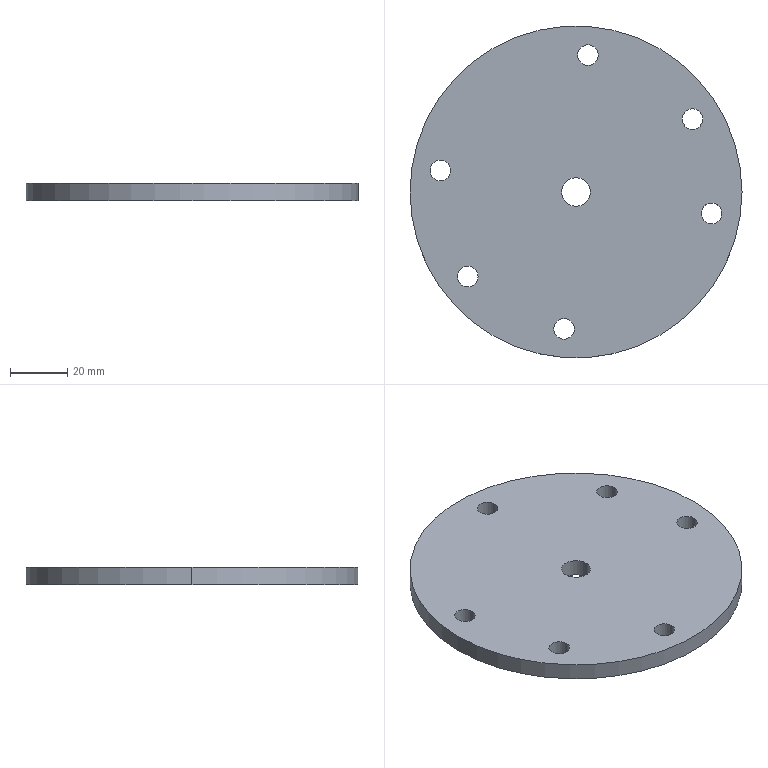Part | SolidWorks | features FlatPattern 1, SMBaseFlange 1, SheetMetal 1 | 1 solid | 18 faces | box 116 x 116 x 6 mm | volume 61473 mm3 | cylinder 16 | plane 2 | commonest cylinder face diameters 7.2 x12 10 x2 116 x2
STEP:
#1=CARTESIAN_POINT('',(-5.,0.,6.));
#2=VERTEX_POINT('',#1);
#3=CARTESIAN_POINT('',(5.,0.,6.));
#4=VERTEX_POINT('',#3);
#5=CARTESIAN_POINT('',(0.,0.,6.));
#6=DIRECTION('',(0.,0.,1.));
#7=DIRECTION('',(1.,0.,0.));
#8=AXIS2_PLACEMENT_3D('',#5,#6,#7);
#9=CIRCLE('',#8,5.);
#10=EDGE_CURVE('',#2,#4,#9,.T.);
#11=ORIENTED_EDGE('',*,*,#10,.T.);
#12=CARTESIAN_POINT('',(5.,0.,0.));
#13=VERTEX_POINT('',#12);
#14=CARTESIAN_POINT('',(5.,0.,6.));
#15=DIRECTION('',(0.,0.,-1.));
#16=VECTOR('',#15,1000.);
#17=LINE('',#14,#16);
#18=EDGE_CURVE('',#4,#13,#17,.T.);
#19=ORIENTED_EDGE('',*,*,#18,.T.);
#20=CARTESIAN_POINT('',(-5.,0.,0.));
#21=VERTEX_POINT('',#20);
#22=CARTESIAN_POINT('',(0.,0.,0.));
#23=DIRECTION('',(0.,0.,1.));
#24=DIRECTION('',(1.,0.,0.));
#25=AXIS2_PLACEMENT_3D('',#22,#23,#24);
#26=CIRCLE('',#25,5.);
#27=EDGE_CURVE('',#21,#13,#26,.T.);
#28=ORIENTED_EDGE('',*,*,#27,.F.);
#29=CARTESIAN_POINT('',(-5.,0.,6.));
#30=DIRECTION('',(0.,0.,-1.));
#31=VECTOR('',#30,1000.);
#32=LINE('',#29,#31);
#33=EDGE_CURVE('',#2,#21,#32,.T.);
#34=ORIENTED_EDGE('',*,*,#33,.F.);
#35=EDGE_LOOP('',(#11,#19,#28,#34));
#36=FACE_OUTER_BOUND('',#35,.T.);
#37=CARTESIAN_POINT('',(0.,0.,6.));
#38=DIRECTION('',(0.,0.,-1.));
#39=DIRECTION('',(-1.,0.,0.));
#40=AXIS2_PLACEMENT_3D('',#37,#38,#39);
#41=CYLINDRICAL_SURFACE('',#40,5.);
#42=ADVANCED_FACE('',(#36),#41,.F.);
#43=CARTESIAN_POINT('',(-7.783,-47.817,6.));
#44=VERTEX_POINT('',#43);
#45=CARTESIAN_POINT('',(-0.5835,-47.817,6.));
#46=VERTEX_POINT('',#45);
#47=CARTESIAN_POINT('',(-4.183,-47.817,6.));
#48=DIRECTION('',(0.,0.,1.));
#49=DIRECTION('',(1.,0.,0.));
#50=AXIS2_PLACEMENT_3D('',#47,#48,#49);
#51=CIRCLE('',#50,3.6);
#52=EDGE_CURVE('',#44,#46,#51,.T.);
#53=ORIENTED_EDGE('',*,*,#52,.T.);
#54=CARTESIAN_POINT('',(-0.5835,-47.817,0.));
#55=VERTEX_POINT('',#54);
#56=CARTESIAN_POINT('',(-0.5835,-47.817,6.));
#57=DIRECTION('',(0.,0.,-1.));
#58=VECTOR('',#57,1000.);
#59=LINE('',#56,#58);
#60=EDGE_CURVE('',#46,#55,#59,.T.);
#61=ORIENTED_EDGE('',*,*,#60,.T.);
#62=CARTESIAN_POINT('',(-7.783,-47.817,0.));
#63=VERTEX_POINT('',#62);
#64=CARTESIAN_POINT('',(-4.183,-47.817,0.));
#65=DIRECTION('',(0.,0.,1.));
#66=DIRECTION('',(1.,0.,0.));
#67=AXIS2_PLACEMENT_3D('',#64,#65,#66);
#68=CIRCLE('',#67,3.6);
#69=EDGE_CURVE('',#63,#55,#68,.T.);
#70=ORIENTED_EDGE('',*,*,#69,.F.);
#71=CARTESIAN_POINT('',(-7.783,-47.817,6.));
#72=DIRECTION('',(0.,0.,-1.));
#73=VECTOR('',#72,1000.);
#74=LINE('',#71,#73);
#75=EDGE_CURVE('',#44,#63,#74,.T.);
#76=ORIENTED_EDGE('',*,*,#75,.F.);
#77=EDGE_LOOP('',(#53,#61,#70,#76));
#78=FACE_OUTER_BOUND('',#77,.T.);
#79=CARTESIAN_POINT('',(-4.183,-47.817,6.));
#80=DIRECTION('',(0.,0.,-1.));
#81=DIRECTION('',(-1.,0.,0.));
#82=AXIS2_PLACEMENT_3D('',#79,#80,#81);
#83=CYLINDRICAL_SURFACE('',#82,3.6);
#84=ADVANCED_FACE('',(#78),#83,.F.);
#85=CARTESIAN_POINT('',(43.809,-7.509,6.));
#86=VERTEX_POINT('',#85);
#87=CARTESIAN_POINT('',(51.009,-7.509,6.));
#88=VERTEX_POINT('',#87);
#89=CARTESIAN_POINT('',(47.409,-7.509,6.));
#90=DIRECTION('',(0.,0.,1.));
#91=DIRECTION('',(1.,0.,0.));
#92=AXIS2_PLACEMENT_3D('',#89,#90,#91);
#93=CIRCLE('',#92,3.6);
#94=EDGE_CURVE('',#86,#88,#93,.T.);
#95=ORIENTED_EDGE('',*,*,#94,.T.);
#96=CARTESIAN_POINT('',(51.009,-7.509,0.));
#97=VERTEX_POINT('',#96);
#98=CARTESIAN_POINT('',(51.009,-7.509,6.));
#99=DIRECTION('',(0.,0.,-1.));
#100=VECTOR('',#99,1000.);
#101=LINE('',#98,#100);
#102=EDGE_CURVE('',#88,#97,#101,.T.);
#103=ORIENTED_EDGE('',*,*,#102,.T.);
#104=CARTESIAN_POINT('',(43.809,-7.509,0.));
#105=VERTEX_POINT('',#104);
#106=CARTESIAN_POINT('',(47.409,-7.509,0.));
#107=DIRECTION('',(0.,0.,1.));
#108=DIRECTION('',(1.,0.,0.));
#109=AXIS2_PLACEMENT_3D('',#106,#107,#108);
#110=CIRCLE('',#109,3.6);
#111=EDGE_CURVE('',#105,#97,#110,.T.);
#112=ORIENTED_EDGE('',*,*,#111,.F.);
#113=CARTESIAN_POINT('',(43.809,-7.509,6.));
#114=DIRECTION('',(0.,0.,-1.));
#115=VECTOR('',#114,1000.);
#116=LINE('',#113,#115);
#117=EDGE_CURVE('',#86,#105,#116,.T.);
#118=ORIENTED_EDGE('',*,*,#117,.F.);
#119=EDGE_LOOP('',(#95,#103,#112,#118));
#120=FACE_OUTER_BOUND('',#119,.T.);
#121=CARTESIAN_POINT('',(47.409,-7.509,6.));
#122=DIRECTION('',(0.,0.,-1.));
#123=DIRECTION('',(-1.,0.,0.));
#124=AXIS2_PLACEMENT_3D('',#121,#122,#123);
#125=CYLINDRICAL_SURFACE('',#124,3.6);
#126=ADVANCED_FACE('',(#120),#125,.F.);
#127=CARTESIAN_POINT('',(37.106,25.436,6.));
#128=VERTEX_POINT('',#127);
#129=CARTESIAN_POINT('',(44.306,25.436,6.));
#130=VERTEX_POINT('',#129);
#131=CARTESIAN_POINT('',(40.706,25.436,6.));
#132=DIRECTION('',(0.,0.,1.));
#133=DIRECTION('',(1.,0.,0.));
#134=AXIS2_PLACEMENT_3D('',#131,#132,#133);
#135=CIRCLE('',#134,3.6);
#136=EDGE_CURVE('',#128,#130,#135,.T.);
#137=ORIENTED_EDGE('',*,*,#136,.T.);
#138=CARTESIAN_POINT('',(44.306,25.436,0.));
#139=VERTEX_POINT('',#138);
#140=CARTESIAN_POINT('',(44.306,25.436,6.));
#141=DIRECTION('',(0.,0.,-1.));
#142=VECTOR('',#141,1000.);
#143=LINE('',#140,#142);
#144=EDGE_CURVE('',#130,#139,#143,.T.);
#145=ORIENTED_EDGE('',*,*,#144,.T.);
#146=CARTESIAN_POINT('',(37.106,25.436,0.));
#147=VERTEX_POINT('',#146);
#148=CARTESIAN_POINT('',(40.706,25.436,0.));
#149=DIRECTION('',(0.,0.,1.));
#150=DIRECTION('',(1.,0.,0.));
#151=AXIS2_PLACEMENT_3D('',#148,#149,#150);
#152=CIRCLE('',#151,3.6);
#153=EDGE_CURVE('',#147,#139,#152,.T.);
#154=ORIENTED_EDGE('',*,*,#153,.F.);
#155=CARTESIAN_POINT('',(37.106,25.436,6.));
#156=DIRECTION('',(0.,0.,-1.));
#157=VECTOR('',#156,1000.);
#158=LINE('',#155,#157);
#159=EDGE_CURVE('',#128,#147,#158,.T.);
#160=ORIENTED_EDGE('',*,*,#159,.F.);
#161=EDGE_LOOP('',(#137,#145,#154,#160));
#162=FACE_OUTER_BOUND('',#161,.T.);
#163=CARTESIAN_POINT('',(40.706,25.436,6.));
#164=DIRECTION('',(0.,0.,-1.));
#165=DIRECTION('',(-1.,0.,0.));
#166=AXIS2_PLACEMENT_3D('',#163,#164,#165);
#167=CYLINDRICAL_SURFACE('',#166,3.6);
#168=ADVANCED_FACE('',(#162),#167,.F.);
#169=CARTESIAN_POINT('',(0.5835,47.817,6.));
#170=VERTEX_POINT('',#169);
#171=CARTESIAN_POINT('',(7.783,47.817,6.));
#172=VERTEX_POINT('',#171);
#173=CARTESIAN_POINT('',(4.183,47.817,6.));
#174=DIRECTION('',(0.,0.,1.));
#175=DIRECTION('',(1.,0.,0.));
#176=AXIS2_PLACEMENT_3D('',#173,#174,#175);
#177=CIRCLE('',#176,3.6);
#178=EDGE_CURVE('',#170,#172,#177,.T.);
#179=ORIENTED_EDGE('',*,*,#178,.T.);
#180=CARTESIAN_POINT('',(7.783,47.817,0.));
#181=VERTEX_POINT('',#180);
#182=CARTESIAN_POINT('',(7.783,47.817,6.));
#183=DIRECTION('',(0.,0.,-1.));
#184=VECTOR('',#183,1000.);
#185=LINE('',#182,#184);
#186=EDGE_CURVE('',#172,#181,#185,.T.);
#187=ORIENTED_EDGE('',*,*,#186,.T.);
#188=CARTESIAN_POINT('',(0.5835,47.817,0.));
#189=VERTEX_POINT('',#188);
#190=CARTESIAN_POINT('',(4.183,47.817,0.));
#191=DIRECTION('',(0.,0.,1.));
#192=DIRECTION('',(1.,0.,0.));
#193=AXIS2_PLACEMENT_3D('',#190,#191,#192);
#194=CIRCLE('',#193,3.6);
#195=EDGE_CURVE('',#189,#181,#194,.T.);
#196=ORIENTED_EDGE('',*,*,#195,.F.);
#197=CARTESIAN_POINT('',(0.5835,47.817,6.));
#198=DIRECTION('',(0.,0.,-1.));
#199=VECTOR('',#198,1000.);
#200=LINE('',#197,#199);
#201=EDGE_CURVE('',#170,#189,#200,.T.);
#202=ORIENTED_EDGE('',*,*,#201,.F.);
#203=EDGE_LOOP('',(#179,#187,#196,#202));
#204=FACE_OUTER_BOUND('',#203,.T.);
#205=CARTESIAN_POINT('',(4.183,47.817,6.));
#206=DIRECTION('',(0.,0.,-1.));
#207=DIRECTION('',(-1.,0.,0.));
#208=AXIS2_PLACEMENT_3D('',#205,#206,#207);
#209=CYLINDRICAL_SURFACE('',#208,3.6);
#210=ADVANCED_FACE('',(#204),#209,.F.);
#211=CARTESIAN_POINT('',(-51.009,7.509,6.));
#212=VERTEX_POINT('',#211);
#213=CARTESIAN_POINT('',(-43.809,7.509,6.));
#214=VERTEX_POINT('',#213);
#215=CARTESIAN_POINT('',(-47.409,7.509,6.));
#216=DIRECTION('',(0.,0.,1.));
#217=DIRECTION('',(1.,0.,0.));
#218=AXIS2_PLACEMENT_3D('',#215,#216,#217);
#219=CIRCLE('',#218,3.6);
#220=EDGE_CURVE('',#212,#214,#219,.T.);
#221=ORIENTED_EDGE('',*,*,#220,.T.);
#222=CARTESIAN_POINT('',(-43.809,7.509,0.));
#223=VERTEX_POINT('',#222);
#224=CARTESIAN_POINT('',(-43.809,7.509,6.));
#225=DIRECTION('',(0.,0.,-1.));
#226=VECTOR('',#225,1000.);
#227=LINE('',#224,#226);
#228=EDGE_CURVE('',#214,#223,#227,.T.);
#229=ORIENTED_EDGE('',*,*,#228,.T.);
#230=CARTESIAN_POINT('',(-51.009,7.509,0.));
#231=VERTEX_POINT('',#230);
#232=CARTESIAN_POINT('',(-47.409,7.509,0.));
#233=DIRECTION('',(0.,0.,1.));
#234=DIRECTION('',(1.,0.,0.));
#235=AXIS2_PLACEMENT_3D('',#232,#233,#234);
#236=CIRCLE('',#235,3.6);
#237=EDGE_CURVE('',#231,#223,#236,.T.);
#238=ORIENTED_EDGE('',*,*,#237,.F.);
#239=CARTESIAN_POINT('',(-51.009,7.509,6.));
#240=DIRECTION('',(0.,0.,-1.));
#241=VECTOR('',#240,1000.);
#242=LINE('',#239,#241);
#243=EDGE_CURVE('',#212,#231,#242,.T.);
#244=ORIENTED_EDGE('',*,*,#243,.F.);
#245=EDGE_LOOP('',(#221,#229,#238,#244));
#246=FACE_OUTER_BOUND('',#245,.T.);
#247=CARTESIAN_POINT('',(-47.409,7.509,6.));
#248=DIRECTION('',(0.,0.,-1.));
#249=DIRECTION('',(-1.,0.,0.));
#250=AXIS2_PLACEMENT_3D('',#247,#248,#249);
#251=CYLINDRICAL_SURFACE('',#250,3.6);
#252=ADVANCED_FACE('',(#246),#251,.F.);
#253=CARTESIAN_POINT('',(-41.425,-29.552,6.));
#254=VERTEX_POINT('',#253);
#255=CARTESIAN_POINT('',(-34.225,-29.552,6.));
#256=VERTEX_POINT('',#255);
#257=CARTESIAN_POINT('',(-37.825,-29.552,6.));
#258=DIRECTION('',(0.,0.,1.));
#259=DIRECTION('',(1.,0.,0.));
#260=AXIS2_PLACEMENT_3D('',#257,#258,#259);
#261=CIRCLE('',#260,3.6);
#262=EDGE_CURVE('',#254,#256,#261,.T.);
#263=ORIENTED_EDGE('',*,*,#262,.T.);
#264=CARTESIAN_POINT('',(-34.225,-29.552,0.));
#265=VERTEX_POINT('',#264);
#266=CARTESIAN_POINT('',(-34.225,-29.552,6.));
#267=DIRECTION('',(0.,0.,-1.));
#268=VECTOR('',#267,1000.);
#269=LINE('',#266,#268);
#270=EDGE_CURVE('',#256,#265,#269,.T.);
#271=ORIENTED_EDGE('',*,*,#270,.T.);
#272=CARTESIAN_POINT('',(-41.425,-29.552,0.));
#273=VERTEX_POINT('',#272);
#274=CARTESIAN_POINT('',(-37.825,-29.552,0.));
#275=DIRECTION('',(0.,0.,1.));
#276=DIRECTION('',(1.,0.,0.));
#277=AXIS2_PLACEMENT_3D('',#274,#275,#276);
#278=CIRCLE('',#277,3.6);
#279=EDGE_CURVE('',#273,#265,#278,.T.);
#280=ORIENTED_EDGE('',*,*,#279,.F.);
#281=CARTESIAN_POINT('',(-41.425,-29.552,6.));
#282=DIRECTION('',(0.,0.,-1.));
#283=VECTOR('',#282,1000.);
#284=LINE('',#281,#283);
#285=EDGE_CURVE('',#254,#273,#284,.T.);
#286=ORIENTED_EDGE('',*,*,#285,.F.);
#287=EDGE_LOOP('',(#263,#271,#280,#286));
#288=FACE_OUTER_BOUND('',#287,.T.);
#289=CARTESIAN_POINT('',(-37.825,-29.552,6.));
#290=DIRECTION('',(0.,0.,-1.));
#291=DIRECTION('',(-1.,0.,0.));
#292=AXIS2_PLACEMENT_3D('',#289,#290,#291);
#293=CYLINDRICAL_SURFACE('',#292,3.6);
#294=ADVANCED_FACE('',(#288),#293,.F.);
#295=CARTESIAN_POINT('',(58.,0.,6.));
#296=VERTEX_POINT('',#295);
#297=CARTESIAN_POINT('',(-58.,0.,6.));
#298=VERTEX_POINT('',#297);
#299=CARTESIAN_POINT('',(0.,0.,6.));
#300=DIRECTION('',(0.,0.,1.));
#301=DIRECTION('',(1.,0.,0.));
#302=AXIS2_PLACEMENT_3D('',#299,#300,#301);
#303=CIRCLE('',#302,58.);
#304=EDGE_CURVE('',#296,#298,#303,.T.);
#305=ORIENTED_EDGE('',*,*,#304,.F.);
#306=CARTESIAN_POINT('',(58.,0.,0.));
#307=VERTEX_POINT('',#306);
#308=CARTESIAN_POINT('',(58.,0.,6.));
#309=DIRECTION('',(0.,0.,-1.));
#310=VECTOR('',#309,1000.);
#311=LINE('',#308,#310);
#312=EDGE_CURVE('',#296,#307,#311,.T.);
#313=ORIENTED_EDGE('',*,*,#312,.T.);
#314=CARTESIAN_POINT('',(-58.,0.,0.));
#315=VERTEX_POINT('',#314);
#316=CARTESIAN_POINT('',(0.,0.,0.));
#317=DIRECTION('',(0.,0.,1.));
#318=DIRECTION('',(1.,0.,0.));
#319=AXIS2_PLACEMENT_3D('',#316,#317,#318);
#320=CIRCLE('',#319,58.);
#321=EDGE_CURVE('',#307,#315,#320,.T.);
#322=ORIENTED_EDGE('',*,*,#321,.T.);
#323=CARTESIAN_POINT('',(-58.,0.,6.));
#324=DIRECTION('',(0.,0.,-1.));
#325=VECTOR('',#324,1000.);
#326=LINE('',#323,#325);
#327=EDGE_CURVE('',#298,#315,#326,.T.);
#328=ORIENTED_EDGE('',*,*,#327,.F.);
#329=EDGE_LOOP('',(#305,#313,#322,#328));
#330=FACE_OUTER_BOUND('',#329,.T.);
#331=CARTESIAN_POINT('',(0.,0.,6.));
#332=DIRECTION('',(0.,0.,-1.));
#333=DIRECTION('',(-1.,0.,0.));
#334=AXIS2_PLACEMENT_3D('',#331,#332,#333);
#335=CYLINDRICAL_SURFACE('',#334,58.);
#336=ADVANCED_FACE('',(#330),#335,.T.);
#337=ORIENTED_EDGE('',*,*,#52,.F.);
#338=CARTESIAN_POINT('',(-4.183,-47.817,6.));
#339=DIRECTION('',(0.,0.,1.));
#340=DIRECTION('',(1.,0.,0.));
#341=AXIS2_PLACEMENT_3D('',#338,#339,#340);
#342=CIRCLE('',#341,3.6);
#343=EDGE_CURVE('',#46,#44,#342,.T.);
#344=ORIENTED_EDGE('',*,*,#343,.F.);
#345=EDGE_LOOP('',(#337,#344));
#346=FACE_BOUND('',#345,.T.);
#347=ORIENTED_EDGE('',*,*,#136,.F.);
#348=CARTESIAN_POINT('',(40.706,25.436,6.));
#349=DIRECTION('',(0.,0.,1.));
#350=DIRECTION('',(1.,0.,0.));
#351=AXIS2_PLACEMENT_3D('',#348,#349,#350);
#352=CIRCLE('',#351,3.6);
#353=EDGE_CURVE('',#130,#128,#352,.T.);
#354=ORIENTED_EDGE('',*,*,#353,.F.);
#355=EDGE_LOOP('',(#347,#354));
#356=FACE_BOUND('',#355,.T.);
#357=ORIENTED_EDGE('',*,*,#220,.F.);
#358=CARTESIAN_POINT('',(-47.409,7.509,6.));
#359=DIRECTION('',(0.,0.,1.));
#360=DIRECTION('',(1.,0.,0.));
#361=AXIS2_PLACEMENT_3D('',#358,#359,#360);
#362=CIRCLE('',#361,3.6);
#363=EDGE_CURVE('',#214,#212,#362,.T.);
#364=ORIENTED_EDGE('',*,*,#363,.F.);
#365=EDGE_LOOP('',(#357,#364));
#366=FACE_BOUND('',#365,.T.);
#367=CARTESIAN_POINT('',(0.,0.,6.));
#368=DIRECTION('',(0.,0.,1.));
#369=DIRECTION('',(1.,0.,0.));
#370=AXIS2_PLACEMENT_3D('',#367,#368,#369);
#371=CIRCLE('',#370,58.);
#372=EDGE_CURVE('',#298,#296,#371,.T.);
#373=ORIENTED_EDGE('',*,*,#372,.T.);
#374=ORIENTED_EDGE('',*,*,#304,.T.);
#375=EDGE_LOOP('',(#373,#374));
#376=FACE_OUTER_BOUND('',#375,.T.);
#377=ORIENTED_EDGE('',*,*,#262,.F.);
#378=CARTESIAN_POINT('',(-37.825,-29.552,6.));
#379=DIRECTION('',(0.,0.,1.));
#380=DIRECTION('',(1.,0.,0.));
#381=AXIS2_PLACEMENT_3D('',#378,#379,#380);
#382=CIRCLE('',#381,3.6);
#383=EDGE_CURVE('',#256,#254,#382,.T.);
#384=ORIENTED_EDGE('',*,*,#383,.F.);
#385=EDGE_LOOP('',(#377,#384));
#386=FACE_BOUND('',#385,.T.);
#387=ORIENTED_EDGE('',*,*,#178,.F.);
#388=CARTESIAN_POINT('',(4.183,47.817,6.));
#389=DIRECTION('',(0.,0.,1.));
#390=DIRECTION('',(1.,0.,0.));
#391=AXIS2_PLACEMENT_3D('',#388,#389,#390);
#392=CIRCLE('',#391,3.6);
#393=EDGE_CURVE('',#172,#170,#392,.T.);
#394=ORIENTED_EDGE('',*,*,#393,.F.);
#395=EDGE_LOOP('',(#387,#394));
#396=FACE_BOUND('',#395,.T.);
#397=ORIENTED_EDGE('',*,*,#94,.F.);
#398=CARTESIAN_POINT('',(47.409,-7.509,6.));
#399=DIRECTION('',(0.,0.,1.));
#400=DIRECTION('',(1.,0.,0.));
#401=AXIS2_PLACEMENT_3D('',#398,#399,#400);
#402=CIRCLE('',#401,3.6);
#403=EDGE_CURVE('',#88,#86,#402,.T.);
#404=ORIENTED_EDGE('',*,*,#403,.F.);
#405=EDGE_LOOP('',(#397,#404));
#406=FACE_BOUND('',#405,.T.);
#407=ORIENTED_EDGE('',*,*,#10,.F.);
#408=CARTESIAN_POINT('',(0.,0.,6.));
#409=DIRECTION('',(0.,0.,1.));
#410=DIRECTION('',(1.,0.,0.));
#411=AXIS2_PLACEMENT_3D('',#408,#409,#410);
#412=CIRCLE('',#411,5.);
#413=EDGE_CURVE('',#4,#2,#412,.T.);
#414=ORIENTED_EDGE('',*,*,#413,.F.);
#415=EDGE_LOOP('',(#407,#414));
#416=FACE_BOUND('',#415,.T.);
#417=CARTESIAN_POINT('',(0.,0.,6.));
#418=DIRECTION('',(0.,0.,1.));
#419=DIRECTION('',(1.,0.,0.));
#420=AXIS2_PLACEMENT_3D('',#417,#418,#419);
#421=PLANE('',#420);
#422=ADVANCED_FACE('',(#346,#356,#366,#376,#386,#396,#406,#416),#421,.T.);
#423=CARTESIAN_POINT('',(0.,0.,0.));
#424=DIRECTION('',(0.,0.,1.));
#425=DIRECTION('',(1.,0.,0.));
#426=AXIS2_PLACEMENT_3D('',#423,#424,#425);
#427=CIRCLE('',#426,58.);
#428=EDGE_CURVE('',#315,#307,#427,.T.);
#429=ORIENTED_EDGE('',*,*,#428,.F.);
#430=ORIENTED_EDGE('',*,*,#321,.F.);
#431=EDGE_LOOP('',(#429,#430));
#432=FACE_OUTER_BOUND('',#431,.T.);
#433=ORIENTED_EDGE('',*,*,#279,.T.);
#434=CARTESIAN_POINT('',(-37.825,-29.552,0.));
#435=DIRECTION('',(0.,0.,1.));
#436=DIRECTION('',(1.,0.,0.));
#437=AXIS2_PLACEMENT_3D('',#434,#435,#436);
#438=CIRCLE('',#437,3.6);
#439=EDGE_CURVE('',#265,#273,#438,.T.);
#440=ORIENTED_EDGE('',*,*,#439,.T.);
#441=EDGE_LOOP('',(#433,#440));
#442=FACE_BOUND('',#441,.T.);
#443=ORIENTED_EDGE('',*,*,#237,.T.);
#444=CARTESIAN_POINT('',(-47.409,7.509,0.));
#445=DIRECTION('',(0.,0.,1.));
#446=DIRECTION('',(1.,0.,0.));
#447=AXIS2_PLACEMENT_3D('',#444,#445,#446);
#448=CIRCLE('',#447,3.6);
#449=EDGE_CURVE('',#223,#231,#448,.T.);
#450=ORIENTED_EDGE('',*,*,#449,.T.);
#451=EDGE_LOOP('',(#443,#450));
#452=FACE_BOUND('',#451,.T.);
#453=ORIENTED_EDGE('',*,*,#195,.T.);
#454=CARTESIAN_POINT('',(4.183,47.817,0.));
#455=DIRECTION('',(0.,0.,1.));
#456=DIRECTION('',(1.,0.,0.));
#457=AXIS2_PLACEMENT_3D('',#454,#455,#456);
#458=CIRCLE('',#457,3.6);
#459=EDGE_CURVE('',#181,#189,#458,.T.);
#460=ORIENTED_EDGE('',*,*,#459,.T.);
#461=EDGE_LOOP('',(#453,#460));
#462=FACE_BOUND('',#461,.T.);
#463=ORIENTED_EDGE('',*,*,#153,.T.);
#464=CARTESIAN_POINT('',(40.706,25.436,0.));
#465=DIRECTION('',(0.,0.,1.));
#466=DIRECTION('',(1.,0.,0.));
#467=AXIS2_PLACEMENT_3D('',#464,#465,#466);
#468=CIRCLE('',#467,3.6);
#469=EDGE_CURVE('',#139,#147,#468,.T.);
#470=ORIENTED_EDGE('',*,*,#469,.T.);
#471=EDGE_LOOP('',(#463,#470));
#472=FACE_BOUND('',#471,.T.);
#473=ORIENTED_EDGE('',*,*,#111,.T.);
#474=CARTESIAN_POINT('',(47.409,-7.509,0.));
#475=DIRECTION('',(0.,0.,1.));
#476=DIRECTION('',(1.,0.,0.));
#477=AXIS2_PLACEMENT_3D('',#474,#475,#476);
#478=CIRCLE('',#477,3.6);
#479=EDGE_CURVE('',#97,#105,#478,.T.);
#480=ORIENTED_EDGE('',*,*,#479,.T.);
#481=EDGE_LOOP('',(#473,#480));
#482=FACE_BOUND('',#481,.T.);
#483=ORIENTED_EDGE('',*,*,#69,.T.);
#484=CARTESIAN_POINT('',(-4.183,-47.817,0.));
#485=DIRECTION('',(0.,0.,1.));
#486=DIRECTION('',(1.,0.,0.));
#487=AXIS2_PLACEMENT_3D('',#484,#485,#486);
#488=CIRCLE('',#487,3.6);
#489=EDGE_CURVE('',#55,#63,#488,.T.);
#490=ORIENTED_EDGE('',*,*,#489,.T.);
#491=EDGE_LOOP('',(#483,#490));
#492=FACE_BOUND('',#491,.T.);
#493=ORIENTED_EDGE('',*,*,#27,.T.);
#494=CARTESIAN_POINT('',(0.,0.,0.));
#495=DIRECTION('',(0.,0.,1.));
#496=DIRECTION('',(1.,0.,0.));
#497=AXIS2_PLACEMENT_3D('',#494,#495,#496);
#498=CIRCLE('',#497,5.);
#499=EDGE_CURVE('',#13,#21,#498,.T.);
#500=ORIENTED_EDGE('',*,*,#499,.T.);
#501=EDGE_LOOP('',(#493,#500));
#502=FACE_BOUND('',#501,.T.);
#503=CARTESIAN_POINT('',(0.,0.,0.));
#504=DIRECTION('',(0.,0.,1.));
#505=DIRECTION('',(1.,0.,0.));
#506=AXIS2_PLACEMENT_3D('',#503,#504,#505);
#507=PLANE('',#506);
#508=ADVANCED_FACE('',(#432,#442,#452,#462,#472,#482,#492,#502),#507,.F.);
#509=ORIENTED_EDGE('',*,*,#312,.F.);
#510=ORIENTED_EDGE('',*,*,#372,.F.);
#511=ORIENTED_EDGE('',*,*,#327,.T.);
#512=ORIENTED_EDGE('',*,*,#428,.T.);
#513=EDGE_LOOP('',(#509,#510,#511,#512));
#514=FACE_OUTER_BOUND('',#513,.T.);
#515=CARTESIAN_POINT('',(0.,0.,6.));
#516=DIRECTION('',(0.,0.,-1.));
#517=DIRECTION('',(-1.,0.,0.));
#518=AXIS2_PLACEMENT_3D('',#515,#516,#517);
#519=CYLINDRICAL_SURFACE('',#518,58.);
#520=ADVANCED_FACE('',(#514),#519,.T.);
#521=ORIENTED_EDGE('',*,*,#270,.F.);
#522=ORIENTED_EDGE('',*,*,#383,.T.);
#523=ORIENTED_EDGE('',*,*,#285,.T.);
#524=ORIENTED_EDGE('',*,*,#439,.F.);
#525=EDGE_LOOP('',(#521,#522,#523,#524));
#526=FACE_OUTER_BOUND('',#525,.T.);
#527=CARTESIAN_POINT('',(-37.825,-29.552,6.));
#528=DIRECTION('',(0.,0.,-1.));
#529=DIRECTION('',(-1.,0.,0.));
#530=AXIS2_PLACEMENT_3D('',#527,#528,#529);
#531=CYLINDRICAL_SURFACE('',#530,3.6);
#532=ADVANCED_FACE('',(#526),#531,.F.);
#533=ORIENTED_EDGE('',*,*,#228,.F.);
#534=ORIENTED_EDGE('',*,*,#363,.T.);
#535=ORIENTED_EDGE('',*,*,#243,.T.);
#536=ORIENTED_EDGE('',*,*,#449,.F.);
#537=EDGE_LOOP('',(#533,#534,#535,#536));
#538=FACE_OUTER_BOUND('',#537,.T.);
#539=CARTESIAN_POINT('',(-47.409,7.509,6.));
#540=DIRECTION('',(0.,0.,-1.));
#541=DIRECTION('',(-1.,0.,0.));
#542=AXIS2_PLACEMENT_3D('',#539,#540,#541);
#543=CYLINDRICAL_SURFACE('',#542,3.6);
#544=ADVANCED_FACE('',(#538),#543,.F.);
#545=ORIENTED_EDGE('',*,*,#186,.F.);
#546=ORIENTED_EDGE('',*,*,#393,.T.);
#547=ORIENTED_EDGE('',*,*,#201,.T.);
#548=ORIENTED_EDGE('',*,*,#459,.F.);
#549=EDGE_LOOP('',(#545,#546,#547,#548));
#550=FACE_OUTER_BOUND('',#549,.T.);
#551=CARTESIAN_POINT('',(4.183,47.817,6.));
#552=DIRECTION('',(0.,0.,-1.));
#553=DIRECTION('',(-1.,0.,0.));
#554=AXIS2_PLACEMENT_3D('',#551,#552,#553);
#555=CYLINDRICAL_SURFACE('',#554,3.6);
#556=ADVANCED_FACE('',(#550),#555,.F.);
#557=ORIENTED_EDGE('',*,*,#144,.F.);
#558=ORIENTED_EDGE('',*,*,#353,.T.);
#559=ORIENTED_EDGE('',*,*,#159,.T.);
#560=ORIENTED_EDGE('',*,*,#469,.F.);
#561=EDGE_LOOP('',(#557,#558,#559,#560));
#562=FACE_OUTER_BOUND('',#561,.T.);
#563=CARTESIAN_POINT('',(40.706,25.436,6.));
#564=DIRECTION('',(0.,0.,-1.));
#565=DIRECTION('',(-1.,0.,0.));
#566=AXIS2_PLACEMENT_3D('',#563,#564,#565);
#567=CYLINDRICAL_SURFACE('',#566,3.6);
#568=ADVANCED_FACE('',(#562),#567,.F.);
#569=ORIENTED_EDGE('',*,*,#102,.F.);
#570=ORIENTED_EDGE('',*,*,#403,.T.);
#571=ORIENTED_EDGE('',*,*,#117,.T.);
#572=ORIENTED_EDGE('',*,*,#479,.F.);
#573=EDGE_LOOP('',(#569,#570,#571,#572));
#574=FACE_OUTER_BOUND('',#573,.T.);
#575=CARTESIAN_POINT('',(47.409,-7.509,6.));
#576=DIRECTION('',(0.,0.,-1.));
#577=DIRECTION('',(-1.,0.,0.));
#578=AXIS2_PLACEMENT_3D('',#575,#576,#577);
#579=CYLINDRICAL_SURFACE('',#578,3.6);
#580=ADVANCED_FACE('',(#574),#579,.F.);
#581=ORIENTED_EDGE('',*,*,#60,.F.);
#582=ORIENTED_EDGE('',*,*,#343,.T.);
#583=ORIENTED_EDGE('',*,*,#75,.T.);
#584=ORIENTED_EDGE('',*,*,#489,.F.);
#585=EDGE_LOOP('',(#581,#582,#583,#584));
#586=FACE_OUTER_BOUND('',#585,.T.);
#587=CARTESIAN_POINT('',(-4.183,-47.817,6.));
#588=DIRECTION('',(0.,0.,-1.));
#589=DIRECTION('',(-1.,0.,0.));
#590=AXIS2_PLACEMENT_3D('',#587,#588,#589);
#591=CYLINDRICAL_SURFACE('',#590,3.6);
#592=ADVANCED_FACE('',(#586),#591,.F.);
#593=ORIENTED_EDGE('',*,*,#18,.F.);
#594=ORIENTED_EDGE('',*,*,#413,.T.);
#595=ORIENTED_EDGE('',*,*,#33,.T.);
#596=ORIENTED_EDGE('',*,*,#499,.F.);
#597=EDGE_LOOP('',(#593,#594,#595,#596));
#598=FACE_OUTER_BOUND('',#597,.T.);
#599=CARTESIAN_POINT('',(0.,0.,6.));
#600=DIRECTION('',(0.,0.,-1.));
#601=DIRECTION('',(-1.,0.,0.));
#602=AXIS2_PLACEMENT_3D('',#599,#600,#601);
#603=CYLINDRICAL_SURFACE('',#602,5.);
#604=ADVANCED_FACE('',(#598),#603,.F.);
#605=CLOSED_SHELL('',(#42,#84,#126,#168,#210,#252,#294,#336,#422,#508,#520,#532,#544,#556,#568,#580,#592,#604));
#606=MANIFOLD_SOLID_BREP('',#605);
#607=CARTESIAN_POINT('',(0.,0.,0.));
#608=DIRECTION('',(0.,0.,1.));
#609=DIRECTION('',(1.,0.,0.));
#610=AXIS2_PLACEMENT_3D('',#607,#608,#609);
#611=(LENGTH_UNIT()NAMED_UNIT(*)SI_UNIT(.MILLI.,.METRE.));
#612=UNCERTAINTY_MEASURE_WITH_UNIT(LENGTH_MEASURE(0.00001),#611,'','');
#613=(NAMED_UNIT(*)PLANE_ANGLE_UNIT()SI_UNIT($,.RADIAN.));
#614=(NAMED_UNIT(*)SI_UNIT($,.STERADIAN.)SOLID_ANGLE_UNIT());
#615=(GEOMETRIC_REPRESENTATION_CONTEXT(3)GLOBAL_UNCERTAINTY_ASSIGNED_CONTEXT((#612))GLOBAL_UNIT_ASSIGNED_CONTEXT((#611,#613,#614))REPRESENTATION_CONTEXT('',''));
#616=ADVANCED_BREP_SHAPE_REPRESENTATION('',(#606,#610),#615);